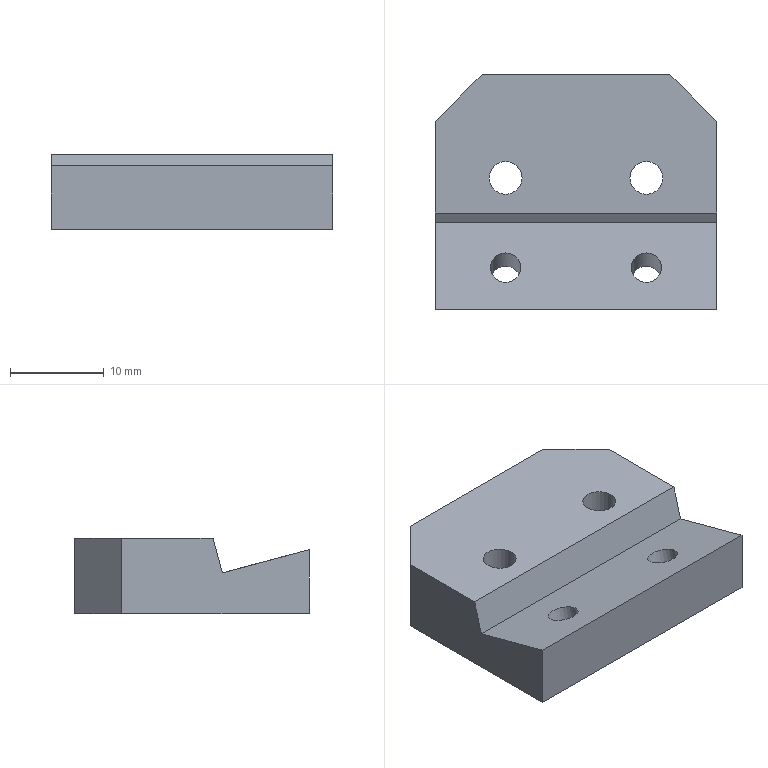Part | NX | 1 solid | 14 faces | box 30 x 25 x 8 mm | volume 4820 mm3 | plane 10 | cylinder 4 | commonest cylinder face diameters 3.242 x2 3.5 x2
STEP:
#1=CARTESIAN_POINT('',(10.,12.5,0.));
#2=VERTEX_POINT('',#1);
#3=CARTESIAN_POINT('',(15.,7.5,0.));
#4=VERTEX_POINT('',#3);
#5=CARTESIAN_POINT('',(12.5,10.,0.));
#6=DIRECTION('',(0.7071,-0.7071,0.));
#7=VECTOR('',#6,1000.);
#8=LINE('',#5,#7);
#9=EDGE_CURVE('',#2,#4,#8,.T.);
#10=ORIENTED_EDGE('',*,*,#9,.T.);
#11=CARTESIAN_POINT('',(15.,7.5,-8.));
#12=VERTEX_POINT('',#11);
#13=CARTESIAN_POINT('',(15.,7.5,-4.));
#14=DIRECTION('',(0.,0.,1.));
#15=VECTOR('',#14,1000.);
#16=LINE('',#13,#15);
#17=EDGE_CURVE('',#12,#4,#16,.T.);
#18=ORIENTED_EDGE('',*,*,#17,.F.);
#19=CARTESIAN_POINT('',(10.,12.5,-8.));
#20=VERTEX_POINT('',#19);
#21=CARTESIAN_POINT('',(12.5,10.,-8.));
#22=DIRECTION('',(0.7071,-0.7071,0.));
#23=VECTOR('',#22,1000.);
#24=LINE('',#21,#23);
#25=EDGE_CURVE('',#20,#12,#24,.T.);
#26=ORIENTED_EDGE('',*,*,#25,.F.);
#27=CARTESIAN_POINT('',(10.,12.5,-4.));
#28=DIRECTION('',(0.,0.,1.));
#29=VECTOR('',#28,1000.);
#30=LINE('',#27,#29);
#31=EDGE_CURVE('',#20,#2,#30,.T.);
#32=ORIENTED_EDGE('',*,*,#31,.T.);
#33=EDGE_LOOP('',(#10,#18,#26,#32));
#34=FACE_BOUND('',#33,.T.);
#35=CARTESIAN_POINT('',(10.,12.5,-4.));
#36=DIRECTION('',(0.7071,0.7071,0.));
#37=DIRECTION('',(0.,0.,1.));
#38=AXIS2_PLACEMENT_3D('',#35,#36,#37);
#39=PLANE('',#38);
#40=ADVANCED_FACE('',(#34),#39,.T.);
#41=ORIENTED_EDGE('',*,*,#31,.F.);
#42=CARTESIAN_POINT('',(-10.,12.5,-8.));
#43=VERTEX_POINT('',#42);
#44=CARTESIAN_POINT('',(0.,12.5,-8.));
#45=DIRECTION('',(1.,0.,0.));
#46=VECTOR('',#45,1000.);
#47=LINE('',#44,#46);
#48=EDGE_CURVE('',#43,#20,#47,.T.);
#49=ORIENTED_EDGE('',*,*,#48,.F.);
#50=CARTESIAN_POINT('',(-10.,12.5,0.));
#51=VERTEX_POINT('',#50);
#52=CARTESIAN_POINT('',(-10.,12.5,-4.));
#53=DIRECTION('',(0.,0.,1.));
#54=VECTOR('',#53,1000.);
#55=LINE('',#52,#54);
#56=EDGE_CURVE('',#43,#51,#55,.T.);
#57=ORIENTED_EDGE('',*,*,#56,.T.);
#58=CARTESIAN_POINT('',(0.,12.5,0.));
#59=DIRECTION('',(1.,0.,0.));
#60=VECTOR('',#59,1000.);
#61=LINE('',#58,#60);
#62=EDGE_CURVE('',#51,#2,#61,.T.);
#63=ORIENTED_EDGE('',*,*,#62,.T.);
#64=EDGE_LOOP('',(#41,#49,#57,#63));
#65=FACE_BOUND('',#64,.T.);
#66=CARTESIAN_POINT('',(-15.,12.5,-8.));
#67=DIRECTION('',(0.,-1.,0.));
#68=DIRECTION('',(1.,0.,0.));
#69=AXIS2_PLACEMENT_3D('',#66,#67,#68);
#70=PLANE('',#69);
#71=ADVANCED_FACE('',(#65),#70,.F.);
#72=CARTESIAN_POINT('',(-9.25,1.5,0.));
#73=VERTEX_POINT('',#72);
#74=CARTESIAN_POINT('',(-7.5,1.5,0.));
#75=DIRECTION('',(0.,0.,1.));
#76=DIRECTION('',(-1.,0.,0.));
#77=AXIS2_PLACEMENT_3D('',#74,#75,#76);
#78=CIRCLE('',#77,1.75);
#79=EDGE_CURVE('',#73,#73,#78,.T.);
#80=ORIENTED_EDGE('',*,*,#79,.F.);
#81=EDGE_LOOP('',(#80));
#82=FACE_BOUND('',#81,.T.);
#83=CARTESIAN_POINT('',(5.75,1.5,0.));
#84=VERTEX_POINT('',#83);
#85=CARTESIAN_POINT('',(7.5,1.5,0.));
#86=DIRECTION('',(0.,0.,1.));
#87=DIRECTION('',(-1.,0.,0.));
#88=AXIS2_PLACEMENT_3D('',#85,#86,#87);
#89=CIRCLE('',#88,1.75);
#90=EDGE_CURVE('',#84,#84,#89,.T.);
#91=ORIENTED_EDGE('',*,*,#90,.F.);
#92=EDGE_LOOP('',(#91));
#93=FACE_BOUND('',#92,.T.);
#94=ORIENTED_EDGE('',*,*,#62,.F.);
#95=CARTESIAN_POINT('',(-15.,7.5,0.));
#96=VERTEX_POINT('',#95);
#97=CARTESIAN_POINT('',(-12.5,10.,0.));
#98=DIRECTION('',(0.7071,0.7071,0.));
#99=VECTOR('',#98,1000.);
#100=LINE('',#97,#99);
#101=EDGE_CURVE('',#96,#51,#100,.T.);
#102=ORIENTED_EDGE('',*,*,#101,.F.);
#103=CARTESIAN_POINT('',(-15.,-2.244,0.));
#104=VERTEX_POINT('',#103);
#105=CARTESIAN_POINT('',(-15.,2.628,0.));
#106=DIRECTION('',(0.,1.,0.));
#107=VECTOR('',#106,1000.);
#108=LINE('',#105,#107);
#109=EDGE_CURVE('',#104,#96,#108,.T.);
#110=ORIENTED_EDGE('',*,*,#109,.F.);
#111=CARTESIAN_POINT('',(15.,-2.244,0.));
#112=VERTEX_POINT('',#111);
#113=CARTESIAN_POINT('',(0.,-2.244,0.));
#114=DIRECTION('',(-1.,0.,0.));
#115=VECTOR('',#114,1000.);
#116=LINE('',#113,#115);
#117=EDGE_CURVE('',#112,#104,#116,.T.);
#118=ORIENTED_EDGE('',*,*,#117,.F.);
#119=CARTESIAN_POINT('',(15.,2.628,0.));
#120=DIRECTION('',(0.,-1.,0.));
#121=VECTOR('',#120,1000.);
#122=LINE('',#119,#121);
#123=EDGE_CURVE('',#4,#112,#122,.T.);
#124=ORIENTED_EDGE('',*,*,#123,.F.);
#125=ORIENTED_EDGE('',*,*,#9,.F.);
#126=EDGE_LOOP('',(#94,#102,#110,#118,#124,#125));
#127=FACE_BOUND('',#126,.T.);
#128=CARTESIAN_POINT('',(0.,0.,0.));
#129=DIRECTION('',(0.,0.,1.));
#130=DIRECTION('',(0.,-1.,0.));
#131=AXIS2_PLACEMENT_3D('',#128,#129,#130);
#132=PLANE('',#131);
#133=ADVANCED_FACE('',(#82,#93,#127),#132,.T.);
#134=CARTESIAN_POINT('',(-9.25,1.5,-8.));
#135=VERTEX_POINT('',#134);
#136=CARTESIAN_POINT('',(-7.5,1.5,-8.));
#137=DIRECTION('',(0.,0.,1.));
#138=DIRECTION('',(-1.,0.,0.));
#139=AXIS2_PLACEMENT_3D('',#136,#137,#138);
#140=CIRCLE('',#139,1.75);
#141=EDGE_CURVE('',#135,#135,#140,.T.);
#142=ORIENTED_EDGE('',*,*,#141,.T.);
#143=EDGE_LOOP('',(#142));
#144=FACE_BOUND('',#143,.T.);
#145=CARTESIAN_POINT('',(5.75,1.5,-8.));
#146=VERTEX_POINT('',#145);
#147=CARTESIAN_POINT('',(7.5,1.5,-8.));
#148=DIRECTION('',(0.,0.,1.));
#149=DIRECTION('',(-1.,0.,0.));
#150=AXIS2_PLACEMENT_3D('',#147,#148,#149);
#151=CIRCLE('',#150,1.75);
#152=EDGE_CURVE('',#146,#146,#151,.T.);
#153=ORIENTED_EDGE('',*,*,#152,.T.);
#154=EDGE_LOOP('',(#153));
#155=FACE_BOUND('',#154,.T.);
#156=CARTESIAN_POINT('',(7.5,-11.242,-8.));
#157=VERTEX_POINT('',#156);
#158=CARTESIAN_POINT('',(7.5,-9.564,-8.));
#159=DIRECTION('',(0.,0.,1.));
#160=DIRECTION('',(0.,-1.,0.));
#161=AXIS2_PLACEMENT_3D('',#158,#159,#160);
#162=ELLIPSE('',#161,1.678,1.621);
#163=EDGE_CURVE('',#157,#157,#162,.F.);
#164=ORIENTED_EDGE('',*,*,#163,.F.);
#165=EDGE_LOOP('',(#164));
#166=FACE_BOUND('',#165,.T.);
#167=CARTESIAN_POINT('',(-7.5,-11.242,-8.));
#168=VERTEX_POINT('',#167);
#169=CARTESIAN_POINT('',(-7.5,-9.564,-8.));
#170=DIRECTION('',(0.,0.,1.));
#171=DIRECTION('',(0.,-1.,0.));
#172=AXIS2_PLACEMENT_3D('',#169,#170,#171);
#173=ELLIPSE('',#172,1.678,1.621);
#174=EDGE_CURVE('',#168,#168,#173,.F.);
#175=ORIENTED_EDGE('',*,*,#174,.F.);
#176=EDGE_LOOP('',(#175));
#177=FACE_BOUND('',#176,.T.);
#178=ORIENTED_EDGE('',*,*,#25,.T.);
#179=CARTESIAN_POINT('',(15.,-12.5,-8.));
#180=VERTEX_POINT('',#179);
#181=CARTESIAN_POINT('',(15.,-2.5,-8.));
#182=DIRECTION('',(0.,-1.,0.));
#183=VECTOR('',#182,1000.);
#184=LINE('',#181,#183);
#185=EDGE_CURVE('',#12,#180,#184,.T.);
#186=ORIENTED_EDGE('',*,*,#185,.T.);
#187=CARTESIAN_POINT('',(-15.,-12.5,-8.));
#188=VERTEX_POINT('',#187);
#189=CARTESIAN_POINT('',(0.,-12.5,-8.));
#190=DIRECTION('',(-1.,0.,0.));
#191=VECTOR('',#190,1000.);
#192=LINE('',#189,#191);
#193=EDGE_CURVE('',#180,#188,#192,.T.);
#194=ORIENTED_EDGE('',*,*,#193,.T.);
#195=CARTESIAN_POINT('',(-15.,7.5,-8.));
#196=VERTEX_POINT('',#195);
#197=CARTESIAN_POINT('',(-15.,-2.5,-8.));
#198=DIRECTION('',(0.,1.,0.));
#199=VECTOR('',#198,1000.);
#200=LINE('',#197,#199);
#201=EDGE_CURVE('',#188,#196,#200,.T.);
#202=ORIENTED_EDGE('',*,*,#201,.T.);
#203=CARTESIAN_POINT('',(-12.5,10.,-8.));
#204=DIRECTION('',(0.7071,0.7071,0.));
#205=VECTOR('',#204,1000.);
#206=LINE('',#203,#205);
#207=EDGE_CURVE('',#196,#43,#206,.T.);
#208=ORIENTED_EDGE('',*,*,#207,.T.);
#209=ORIENTED_EDGE('',*,*,#48,.T.);
#210=EDGE_LOOP('',(#178,#186,#194,#202,#208,#209));
#211=FACE_BOUND('',#210,.T.);
#212=CARTESIAN_POINT('',(0.,0.,-8.));
#213=DIRECTION('',(0.,0.,1.));
#214=DIRECTION('',(0.,-1.,0.));
#215=AXIS2_PLACEMENT_3D('',#212,#213,#214);
#216=PLANE('',#215);
#217=ADVANCED_FACE('',(#144,#155,#166,#177,#211),#216,.F.);
#218=ORIENTED_EDGE('',*,*,#17,.T.);
#219=ORIENTED_EDGE('',*,*,#123,.T.);
#220=CARTESIAN_POINT('',(15.,-3.227,-3.671));
#221=VERTEX_POINT('',#220);
#222=CARTESIAN_POINT('',(15.,-2.735,-1.835));
#223=DIRECTION('',(0.,0.2588,0.9659));
#224=VECTOR('',#223,1000.);
#225=LINE('',#222,#224);
#226=EDGE_CURVE('',#221,#112,#225,.T.);
#227=ORIENTED_EDGE('',*,*,#226,.F.);
#228=CARTESIAN_POINT('',(15.,-12.5,-1.186));
#229=VERTEX_POINT('',#228);
#230=CARTESIAN_POINT('',(15.,-7.864,-2.428));
#231=DIRECTION('',(0.,0.9659,-0.2588));
#232=VECTOR('',#231,1000.);
#233=LINE('',#230,#232);
#234=EDGE_CURVE('',#229,#221,#233,.T.);
#235=ORIENTED_EDGE('',*,*,#234,.F.);
#236=CARTESIAN_POINT('',(15.,-12.5,-4.593));
#237=DIRECTION('',(0.,0.,1.));
#238=VECTOR('',#237,1000.);
#239=LINE('',#236,#238);
#240=EDGE_CURVE('',#180,#229,#239,.T.);
#241=ORIENTED_EDGE('',*,*,#240,.F.);
#242=ORIENTED_EDGE('',*,*,#185,.F.);
#243=EDGE_LOOP('',(#218,#219,#227,#235,#241,#242));
#244=FACE_BOUND('',#243,.T.);
#245=CARTESIAN_POINT('',(15.,12.5,-8.));
#246=DIRECTION('',(-1.,0.,0.));
#247=DIRECTION('',(0.,-1.,0.));
#248=AXIS2_PLACEMENT_3D('',#245,#246,#247);
#249=PLANE('',#248);
#250=ADVANCED_FACE('',(#244),#249,.F.);
#251=ORIENTED_EDGE('',*,*,#101,.T.);
#252=ORIENTED_EDGE('',*,*,#56,.F.);
#253=ORIENTED_EDGE('',*,*,#207,.F.);
#254=CARTESIAN_POINT('',(-15.,7.5,-4.));
#255=DIRECTION('',(0.,0.,1.));
#256=VECTOR('',#255,1000.);
#257=LINE('',#254,#256);
#258=EDGE_CURVE('',#196,#96,#257,.T.);
#259=ORIENTED_EDGE('',*,*,#258,.T.);
#260=EDGE_LOOP('',(#251,#252,#253,#259));
#261=FACE_BOUND('',#260,.T.);
#262=CARTESIAN_POINT('',(-15.,7.5,-4.));
#263=DIRECTION('',(-0.7071,0.7071,0.));
#264=DIRECTION('',(0.,0.,1.));
#265=AXIS2_PLACEMENT_3D('',#262,#263,#264);
#266=PLANE('',#265);
#267=ADVANCED_FACE('',(#261),#266,.T.);
#268=ORIENTED_EDGE('',*,*,#258,.F.);
#269=ORIENTED_EDGE('',*,*,#201,.F.);
#270=CARTESIAN_POINT('',(-15.,-12.5,-1.186));
#271=VERTEX_POINT('',#270);
#272=CARTESIAN_POINT('',(-15.,-12.5,-4.593));
#273=DIRECTION('',(0.,0.,1.));
#274=VECTOR('',#273,1000.);
#275=LINE('',#272,#274);
#276=EDGE_CURVE('',#188,#271,#275,.T.);
#277=ORIENTED_EDGE('',*,*,#276,.T.);
#278=CARTESIAN_POINT('',(-15.,-3.227,-3.671));
#279=VERTEX_POINT('',#278);
#280=CARTESIAN_POINT('',(-15.,-7.864,-2.428));
#281=DIRECTION('',(0.,-0.9659,0.2588));
#282=VECTOR('',#281,1000.);
#283=LINE('',#280,#282);
#284=EDGE_CURVE('',#279,#271,#283,.T.);
#285=ORIENTED_EDGE('',*,*,#284,.F.);
#286=CARTESIAN_POINT('',(-15.,-2.735,-1.835));
#287=DIRECTION('',(0.,-0.2588,-0.9659));
#288=VECTOR('',#287,1000.);
#289=LINE('',#286,#288);
#290=EDGE_CURVE('',#104,#279,#289,.T.);
#291=ORIENTED_EDGE('',*,*,#290,.F.);
#292=ORIENTED_EDGE('',*,*,#109,.T.);
#293=EDGE_LOOP('',(#268,#269,#277,#285,#291,#292));
#294=FACE_BOUND('',#293,.T.);
#295=CARTESIAN_POINT('',(-15.,-12.5,-8.));
#296=DIRECTION('',(1.,0.,0.));
#297=DIRECTION('',(0.,1.,0.));
#298=AXIS2_PLACEMENT_3D('',#295,#296,#297);
#299=PLANE('',#298);
#300=ADVANCED_FACE('',(#294),#299,.F.);
#301=ORIENTED_EDGE('',*,*,#174,.T.);
#302=EDGE_LOOP('',(#301));
#303=FACE_BOUND('',#302,.T.);
#304=CARTESIAN_POINT('',(-7.5,-6.491,-2.796));
#305=VERTEX_POINT('',#304);
#306=CARTESIAN_POINT('',(-7.5,-8.057,-2.376));
#307=DIRECTION('',(0.,0.2588,0.9659));
#308=DIRECTION('',(0.,0.9659,-0.2588));
#309=AXIS2_PLACEMENT_3D('',#306,#307,#308);
#310=CIRCLE('',#309,1.621);
#311=EDGE_CURVE('',#305,#305,#310,.T.);
#312=ORIENTED_EDGE('',*,*,#311,.T.);
#313=EDGE_LOOP('',(#312));
#314=FACE_BOUND('',#313,.T.);
#315=CARTESIAN_POINT('',(-7.5,-8.057,-2.376));
#316=DIRECTION('',(0.,-0.2588,-0.9659));
#317=DIRECTION('',(0.,-0.9659,0.2588));
#318=AXIS2_PLACEMENT_3D('',#315,#316,#317);
#319=CYLINDRICAL_SURFACE('',#318,1.621);
#320=ADVANCED_FACE('',(#303,#314),#319,.F.);
#321=ORIENTED_EDGE('',*,*,#276,.F.);
#322=ORIENTED_EDGE('',*,*,#193,.F.);
#323=ORIENTED_EDGE('',*,*,#240,.T.);
#324=CARTESIAN_POINT('',(0.,-12.5,-1.186));
#325=DIRECTION('',(-1.,0.,0.));
#326=VECTOR('',#325,1000.);
#327=LINE('',#324,#326);
#328=EDGE_CURVE('',#229,#271,#327,.T.);
#329=ORIENTED_EDGE('',*,*,#328,.T.);
#330=EDGE_LOOP('',(#321,#322,#323,#329));
#331=FACE_BOUND('',#330,.T.);
#332=CARTESIAN_POINT('',(15.,-12.5,-8.));
#333=DIRECTION('',(0.,1.,0.));
#334=DIRECTION('',(-1.,0.,0.));
#335=AXIS2_PLACEMENT_3D('',#332,#333,#334);
#336=PLANE('',#335);
#337=ADVANCED_FACE('',(#331),#336,.F.);
#338=ORIENTED_EDGE('',*,*,#79,.T.);
#339=EDGE_LOOP('',(#338));
#340=FACE_BOUND('',#339,.T.);
#341=ORIENTED_EDGE('',*,*,#141,.F.);
#342=EDGE_LOOP('',(#341));
#343=FACE_BOUND('',#342,.T.);
#344=CARTESIAN_POINT('',(-7.5,1.5,-4.));
#345=DIRECTION('',(0.,0.,1.));
#346=DIRECTION('',(0.,-1.,0.));
#347=AXIS2_PLACEMENT_3D('',#344,#345,#346);
#348=CYLINDRICAL_SURFACE('',#347,1.75);
#349=ADVANCED_FACE('',(#340,#343),#348,.F.);
#350=ORIENTED_EDGE('',*,*,#90,.T.);
#351=EDGE_LOOP('',(#350));
#352=FACE_BOUND('',#351,.T.);
#353=ORIENTED_EDGE('',*,*,#152,.F.);
#354=EDGE_LOOP('',(#353));
#355=FACE_BOUND('',#354,.T.);
#356=CARTESIAN_POINT('',(7.5,1.5,-4.));
#357=DIRECTION('',(0.,0.,1.));
#358=DIRECTION('',(0.,-1.,0.));
#359=AXIS2_PLACEMENT_3D('',#356,#357,#358);
#360=CYLINDRICAL_SURFACE('',#359,1.75);
#361=ADVANCED_FACE('',(#352,#355),#360,.F.);
#362=CARTESIAN_POINT('',(0.,-3.227,-3.671));
#363=DIRECTION('',(-1.,0.,0.));
#364=VECTOR('',#363,1000.);
#365=LINE('',#362,#364);
#366=EDGE_CURVE('',#221,#279,#365,.T.);
#367=ORIENTED_EDGE('',*,*,#366,.F.);
#368=ORIENTED_EDGE('',*,*,#226,.T.);
#369=ORIENTED_EDGE('',*,*,#117,.T.);
#370=ORIENTED_EDGE('',*,*,#290,.T.);
#371=EDGE_LOOP('',(#367,#368,#369,#370));
#372=FACE_BOUND('',#371,.T.);
#373=CARTESIAN_POINT('',(15.,-3.227,-3.671));
#374=DIRECTION('',(0.,-0.9659,0.2588));
#375=DIRECTION('',(0.,0.2588,0.9659));
#376=AXIS2_PLACEMENT_3D('',#373,#374,#375);
#377=PLANE('',#376);
#378=ADVANCED_FACE('',(#372),#377,.T.);
#379=CARTESIAN_POINT('',(7.5,-6.491,-2.796));
#380=VERTEX_POINT('',#379);
#381=CARTESIAN_POINT('',(7.5,-8.057,-2.376));
#382=DIRECTION('',(0.,-0.2588,-0.9659));
#383=DIRECTION('',(0.,0.9659,-0.2588));
#384=AXIS2_PLACEMENT_3D('',#381,#382,#383);
#385=CIRCLE('',#384,1.621);
#386=EDGE_CURVE('',#380,#380,#385,.T.);
#387=ORIENTED_EDGE('',*,*,#386,.T.);
#388=EDGE_LOOP('',(#387));
#389=FACE_BOUND('',#388,.T.);
#390=ORIENTED_EDGE('',*,*,#311,.F.);
#391=EDGE_LOOP('',(#390));
#392=FACE_BOUND('',#391,.T.);
#393=ORIENTED_EDGE('',*,*,#234,.T.);
#394=ORIENTED_EDGE('',*,*,#366,.T.);
#395=ORIENTED_EDGE('',*,*,#284,.T.);
#396=ORIENTED_EDGE('',*,*,#328,.F.);
#397=EDGE_LOOP('',(#393,#394,#395,#396));
#398=FACE_BOUND('',#397,.T.);
#399=CARTESIAN_POINT('',(15.,-16.926,0.));
#400=DIRECTION('',(0.,0.2588,0.9659));
#401=DIRECTION('',(0.,0.9659,-0.2588));
#402=AXIS2_PLACEMENT_3D('',#399,#400,#401);
#403=PLANE('',#402);
#404=ADVANCED_FACE('',(#389,#392,#398),#403,.T.);
#405=ORIENTED_EDGE('',*,*,#163,.T.);
#406=EDGE_LOOP('',(#405));
#407=FACE_BOUND('',#406,.T.);
#408=ORIENTED_EDGE('',*,*,#386,.F.);
#409=EDGE_LOOP('',(#408));
#410=FACE_BOUND('',#409,.T.);
#411=CARTESIAN_POINT('',(7.5,-8.057,-2.376));
#412=DIRECTION('',(0.,-0.2588,-0.9659));
#413=DIRECTION('',(0.,-0.9659,0.2588));
#414=AXIS2_PLACEMENT_3D('',#411,#412,#413);
#415=CYLINDRICAL_SURFACE('',#414,1.621);
#416=ADVANCED_FACE('',(#407,#410),#415,.F.);
#417=CLOSED_SHELL('',(#40,#71,#133,#217,#250,#267,#300,#320,#337,#349,#361,#378,#404,#416));
#418=MANIFOLD_SOLID_BREP('',#417);
#419=(LENGTH_UNIT()NAMED_UNIT(*)SI_UNIT(.MILLI.,.METRE.));
#420=UNCERTAINTY_MEASURE_WITH_UNIT(LENGTH_MEASURE(0.00001),#419,'','');
#421=(NAMED_UNIT(*)PLANE_ANGLE_UNIT()SI_UNIT($,.RADIAN.));
#422=(NAMED_UNIT(*)SI_UNIT($,.STERADIAN.)SOLID_ANGLE_UNIT());
#423=(GEOMETRIC_REPRESENTATION_CONTEXT(3)GLOBAL_UNCERTAINTY_ASSIGNED_CONTEXT((#420))GLOBAL_UNIT_ASSIGNED_CONTEXT((#419,#421,#422))REPRESENTATION_CONTEXT('',''));
#424=ADVANCED_BREP_SHAPE_REPRESENTATION('',(#418),#423);